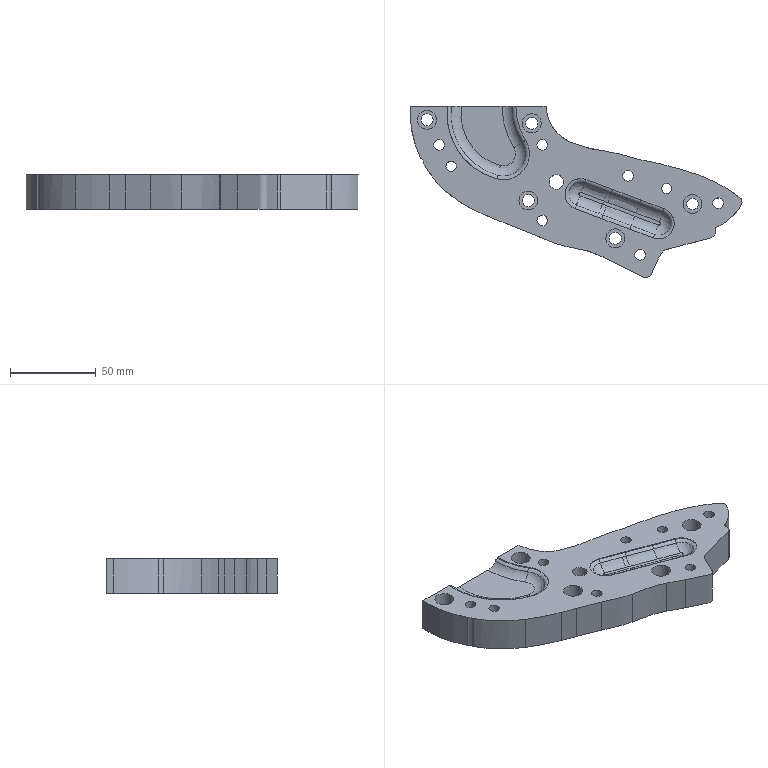Part | NX | features 23 2 | 1 solid | 88 faces | box 193.397 x 99.583 x 20 mm | volume 185252 mm3 | spline 32 | cylinder 30 | plane 18 | torus 8 | commonest cylinder face diameters 6.2 x6 7 x5 11 x5 5 x4 14 x4 6.001 x2